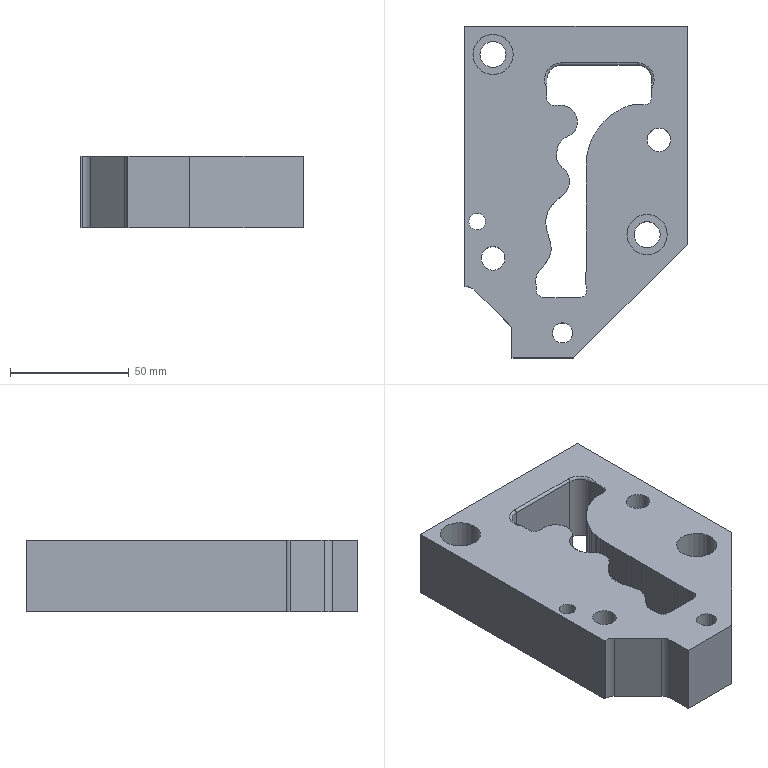Part | STEP file | 1 solid | 202 faces | box 94 x 140 x 30 mm | volume 271163 mm3 | plane 180 | cylinder 20 | torus 2 | commonest cylinder face diameters 6.28 x4 10 x4 11.72 x3 11 x2 12.28 x2 17 x2